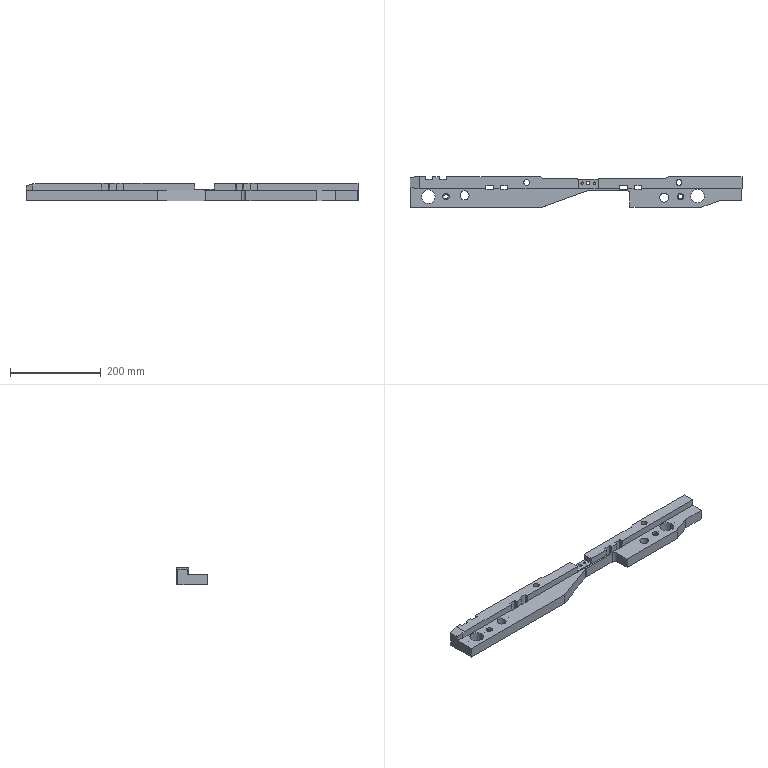Part | STEP file | gslz 2016.10.28-13_id990_x_t | 1 solid | 116 faces | box 730 x 68 x 38 mm | volume 1131774 mm3 | plane 57 | cylinder 47 | cone 12 | commonest cylinder face diameters 2 x22 5.2 x6 6.8 x4 14 x4 10.3 x2 13 x2